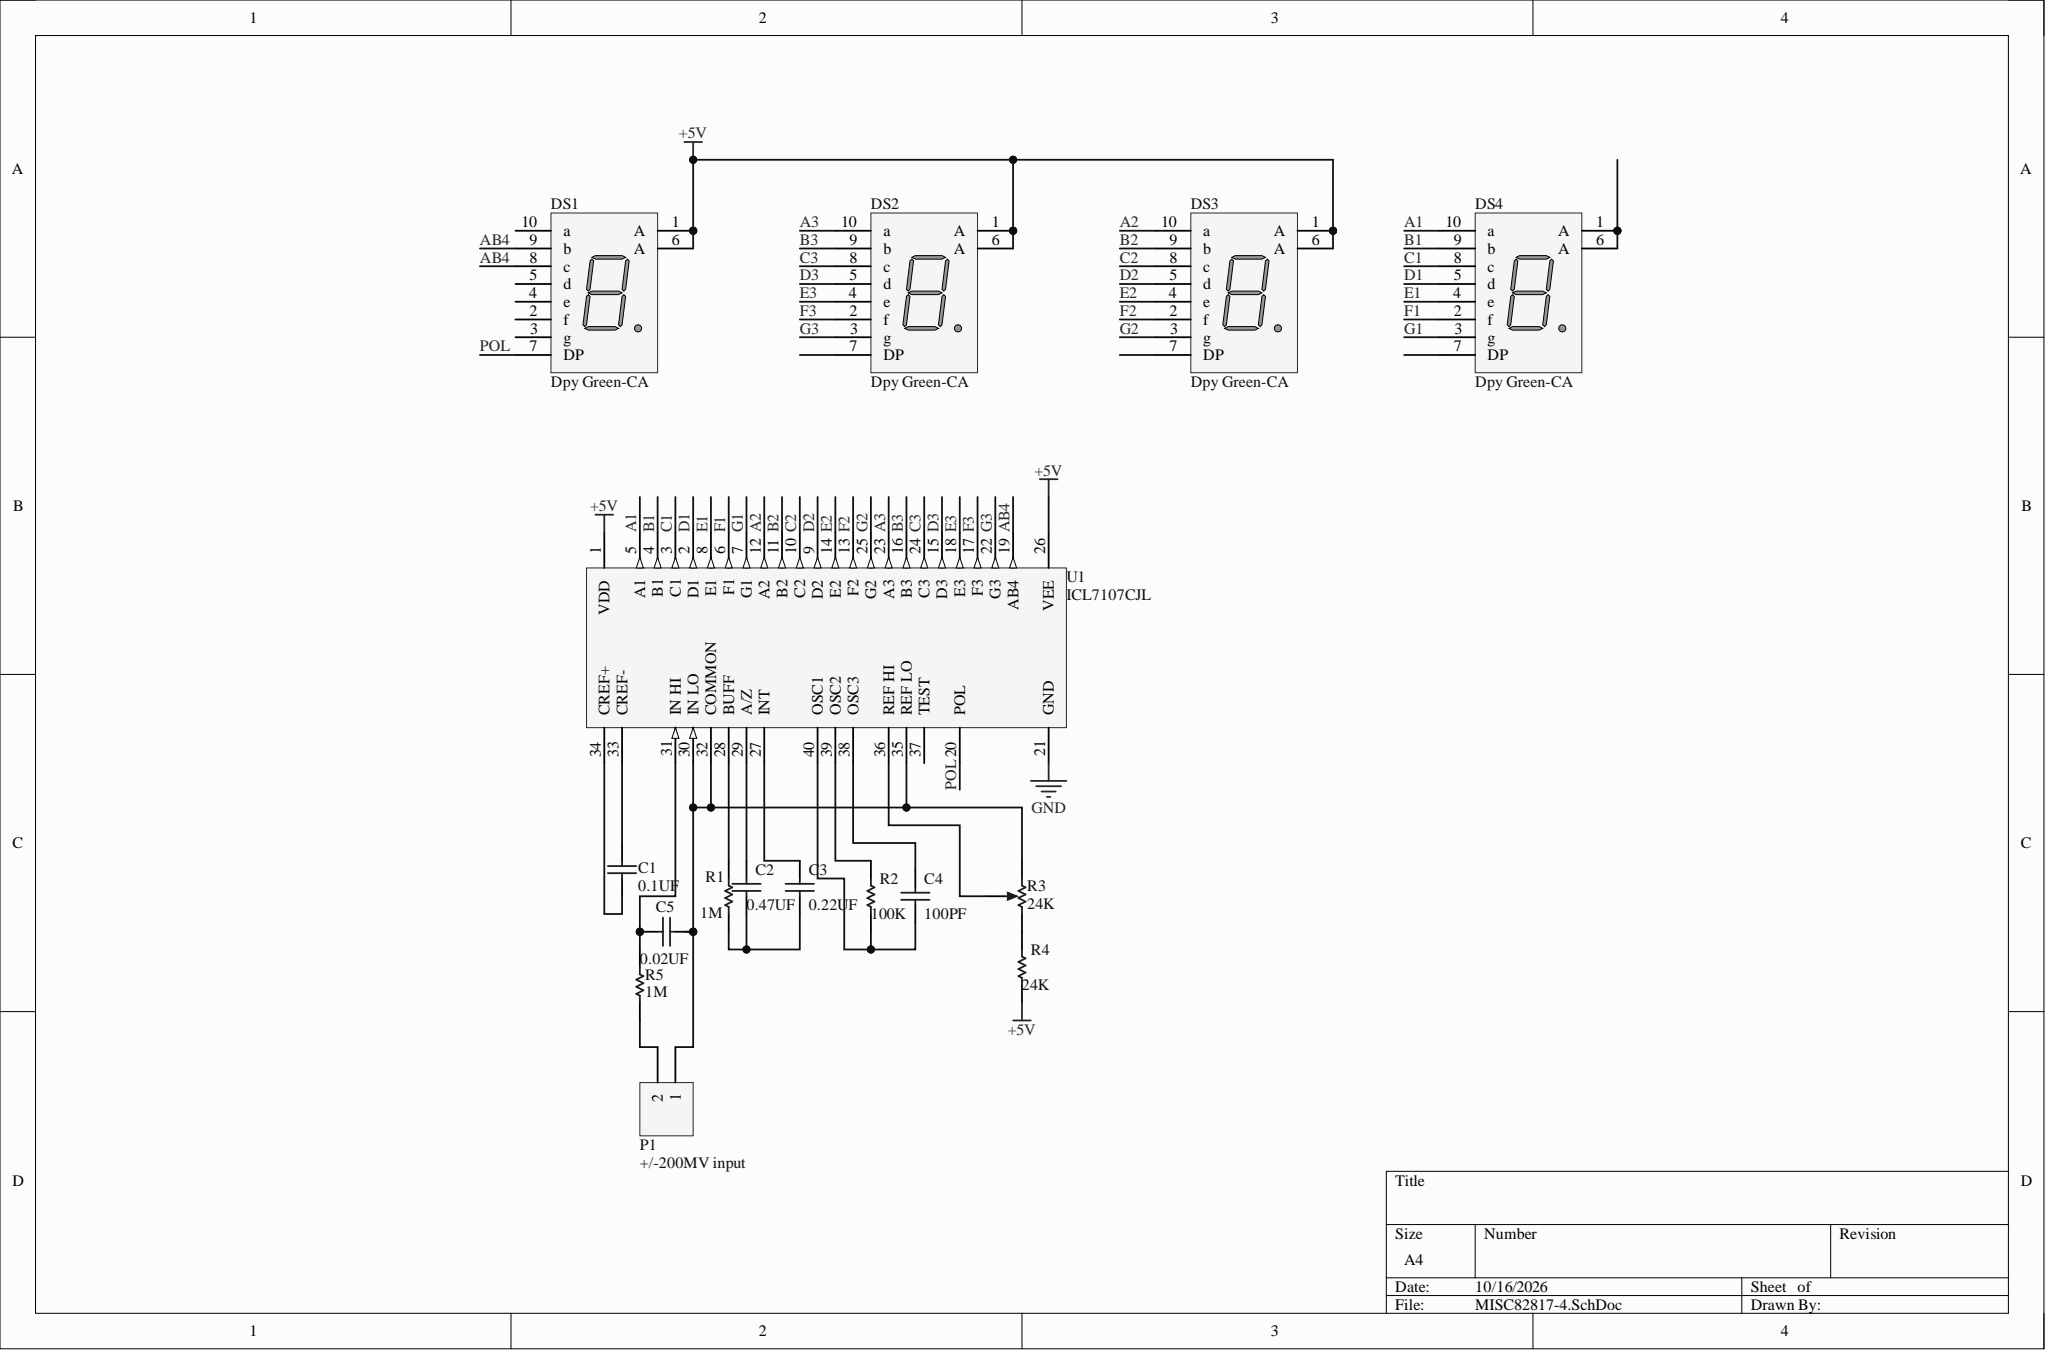Circuit board | Altium Designer | 16 parts | 39 nets
Bill of materials:
Comment,Description,Designator,Footprint,LibRef,Quantity
"0.1UF","Capacitor","C1","RAD-0.3","Cap","1"
"0.47UF","Capacitor","C2","RAD-0.3","Cap","1"
"0.22UF","Capacitor","C3","RAD-0.3","Cap","1"
"100PF","Capacitor","C4","RAD-0.3","Cap","1"
"0.02UF","Capacitor","C5","RAD-0.3","Cap","1"
"Dpy Green-CA","7.62 mm Black Surface Green 7-Segment Display: CA, RH DP","DS1, DS2, DS3, DS4","A","Dpy Green-CA","4"
"+/-200MV input","Header, 2-Pin","P1","HDR1X2","Header 2","1"
"1M","Resistor","R1, R5","AXIAL-0.3","Res1","2"
"100K","Resistor","R2","AXIAL-0.3","Res1","1"
"24K","Potentiometer","R3","VR5","RPot","1"
"24K","Resistor","R4","AXIAL-0.3","Res1","1"
"ICL7107CJL","","U1","JL40A","ICL7107CJL","1"
Netlist (Protel format):
[
C1
RAD-0.3
0.1UF



]
[
C2
RAD-0.3
0.47UF



]
[
C3
RAD-0.3
0.22UF



]
[
C4
RAD-0.3
100PF



]
[
C5
RAD-0.3
0.02UF



]
[
DS1
A
Dpy Green-CA



]
[
DS2
A
Dpy Green-CA



]
[
DS3
A
Dpy Green-CA



]
[
DS4
A
Dpy Green-CA



]
[
P1
HDR1X2
+/-200MV input



]
[
R1
AXIAL-0.3
1M



]
[
R2
AXIAL-0.3
100K



]
[
R3
VR5
24K



]
[
R4
AXIAL-0.3
24K



]
[
R5
AXIAL-0.3
1M



]
[
U1
JL40A
ICL7107CJL



]
(
POL
DS1-7
U1-20
)
(
NetR3_3
R3-3
U1-36
)
(
NetR3_2
R3-2
R4-2
)
(
NetR2_2
R2-2
U1-39
)
(
NetR1_2
R1-2
U1-28
)
(
NetP1_2
P1-2
R5-1
)
(
NetDS4_1
DS4-1
DS4-6
)
(
NetC5_2
C5-2
R5-2
U1-31
)
(
NetC5_1
C5-1
P1-1
R3-1
U1-30
U1-32
U1-35
)
(
NetC4_2
C4-2
R2-1
U1-40
)
(
NetC4_1
C4-1
U1-38
)
(
NetC3_1
C3-1
U1-27
)
(
NetC2_2
C2-2
C3-2
R1-1
)
(
NetC2_1
C2-1
U1-29
)
(
NetC1_2
C1-2
U1-33
)
(
NetC1_1
C1-1
U1-34
)
(
G3
DS2-3
U1-22
)
(
G2
DS3-3
U1-25
)
(
G1
DS4-3
U1-7
)
(
F3
DS2-2
U1-17
)
(
F2
DS3-2
U1-13
)
(
F1
DS4-2
U1-6
)
(
E3
DS2-4
U1-18
)
(
E2
DS3-4
U1-14
)
(
E1
DS4-4
U1-8
)
(
D3
DS2-5
U1-15
)
(
D2
DS3-5
U1-9
)
(
D1
DS4-5
U1-2
)
(
C3
DS2-8
U1-24
)
(
C2
DS3-8
U1-10
)
(
C1
DS4-8
U1-3
)
(
B3
DS2-9
U1-16
)
(
B2
DS3-9
U1-11
)
(
B1
DS4-9
U1-4
)
(
AB4
DS1-8
DS1-9
U1-19
)
(
A3
DS2-10
U1-23
)
(
A2
DS3-10
U1-12
)
(
A1
DS4-10
U1-5
)
(
+5V
DS1-1
DS1-6
DS2-1
DS2-6
DS3-1
DS3-6
R4-1
U1-1
U1-26
)